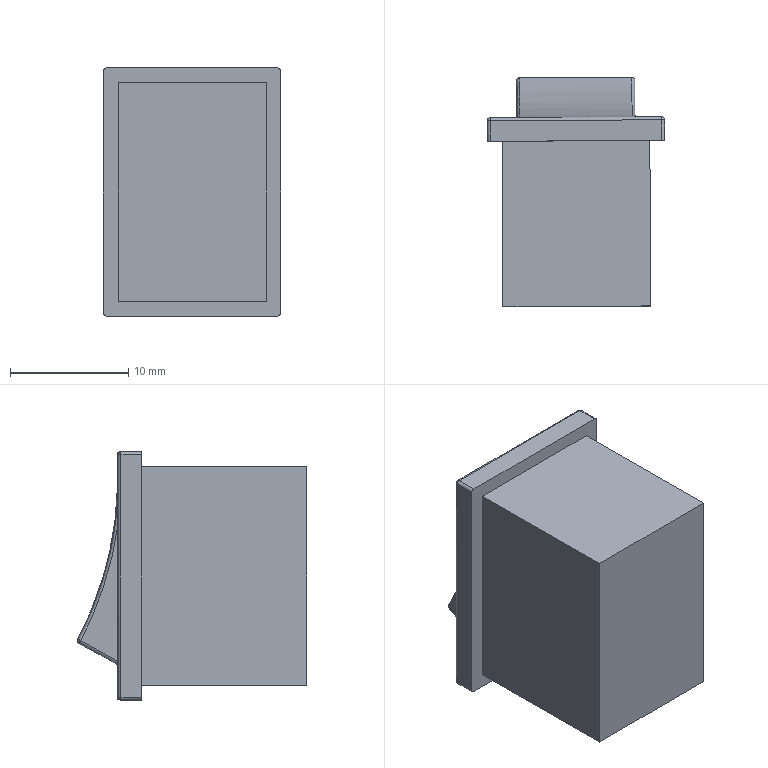Part | SolidWorks | features BaseBody 1 | 1 solid | 36 faces | box 15.007 x 19.46 x 21 mm | volume 4055 mm3 | cylinder 14 | plane 14 | spline 8 | commonest cylinder face diameters 0.5 x13 57.288 x1